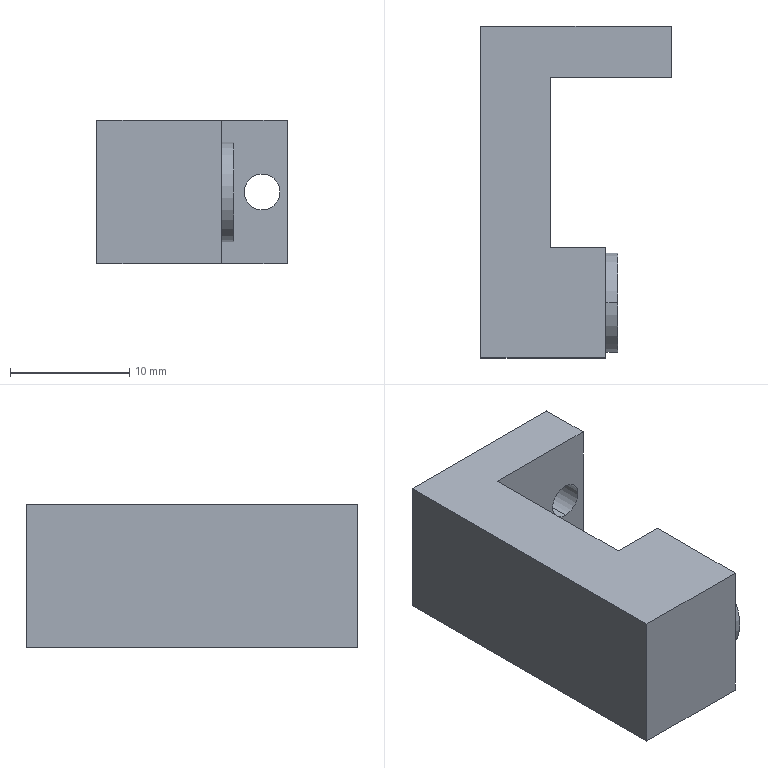Part | SolidWorks | features SavedExtBody 1 | 1 solid | 21 faces | box 15.948 x 27.791 x 12 mm | volume 2925 mm3 | plane 11 | cylinder 8 | cone 2 | commonest cylinder face diameters 3 x4 4.217 x2 8.358 x2
STEP:
#1=CARTESIAN_POINT('',(81.489,-181.285,66.5));
#2=VERTEX_POINT('',#1);
#3=CARTESIAN_POINT('',(81.489,-181.285,63.5));
#4=VERTEX_POINT('',#3);
#5=CARTESIAN_POINT('',(81.489,-181.285,65.));
#6=DIRECTION('',(0.,-1.,0.));
#7=DIRECTION('',(0.,0.,-1.));
#8=AXIS2_PLACEMENT_3D('',#5,#6,#7);
#9=CIRCLE('',#8,1.5);
#10=EDGE_CURVE('',#2,#4,#9,.T.);
#11=ORIENTED_EDGE('',*,*,#10,.F.);
#12=CARTESIAN_POINT('',(81.489,-185.569,66.5));
#13=VERTEX_POINT('',#12);
#14=CARTESIAN_POINT('',(81.489,-163.569,66.5));
#15=DIRECTION('',(0.,-1.,0.));
#16=VECTOR('',#15,1000.);
#17=LINE('',#14,#16);
#18=EDGE_CURVE('',#2,#13,#17,.T.);
#19=ORIENTED_EDGE('',*,*,#18,.T.);
#20=CARTESIAN_POINT('',(81.489,-185.569,63.5));
#21=VERTEX_POINT('',#20);
#22=CARTESIAN_POINT('',(81.489,-185.569,65.));
#23=DIRECTION('',(0.,-1.,0.));
#24=DIRECTION('',(0.,0.,-1.));
#25=AXIS2_PLACEMENT_3D('',#22,#23,#24);
#26=CIRCLE('',#25,1.5);
#27=EDGE_CURVE('',#13,#21,#26,.T.);
#28=ORIENTED_EDGE('',*,*,#27,.T.);
#29=CARTESIAN_POINT('',(81.489,-163.569,63.5));
#30=DIRECTION('',(0.,-1.,0.));
#31=VECTOR('',#30,1000.);
#32=LINE('',#29,#31);
#33=EDGE_CURVE('',#4,#21,#32,.T.);
#34=ORIENTED_EDGE('',*,*,#33,.F.);
#35=EDGE_LOOP('',(#11,#19,#28,#34));
#36=FACE_OUTER_BOUND('',#35,.T.);
#37=CARTESIAN_POINT('',(81.489,-163.569,65.));
#38=DIRECTION('',(0.,-1.,0.));
#39=DIRECTION('',(0.,0.,-1.));
#40=AXIS2_PLACEMENT_3D('',#37,#38,#39);
#41=CYLINDRICAL_SURFACE('',#40,1.5);
#42=ADVANCED_FACE('',(#36),#41,.F.);
#43=CARTESIAN_POINT('',(87.424,-181.285,66.5));
#44=VERTEX_POINT('',#43);
#45=CARTESIAN_POINT('',(87.424,-181.285,63.5));
#46=VERTEX_POINT('',#45);
#47=CARTESIAN_POINT('',(87.424,-181.285,65.));
#48=DIRECTION('',(0.,-1.,0.));
#49=DIRECTION('',(0.,0.,-1.));
#50=AXIS2_PLACEMENT_3D('',#47,#48,#49);
#51=CIRCLE('',#50,1.5);
#52=EDGE_CURVE('',#44,#46,#51,.T.);
#53=ORIENTED_EDGE('',*,*,#52,.F.);
#54=CARTESIAN_POINT('',(87.424,-185.569,66.5));
#55=VERTEX_POINT('',#54);
#56=CARTESIAN_POINT('',(87.424,-163.569,66.5));
#57=DIRECTION('',(0.,-1.,0.));
#58=VECTOR('',#57,1000.);
#59=LINE('',#56,#58);
#60=EDGE_CURVE('',#44,#55,#59,.T.);
#61=ORIENTED_EDGE('',*,*,#60,.T.);
#62=CARTESIAN_POINT('',(87.424,-185.569,63.5));
#63=VERTEX_POINT('',#62);
#64=CARTESIAN_POINT('',(87.424,-185.569,65.));
#65=DIRECTION('',(0.,-1.,0.));
#66=DIRECTION('',(0.,0.,1.));
#67=AXIS2_PLACEMENT_3D('',#64,#65,#66);
#68=CIRCLE('',#67,1.5);
#69=EDGE_CURVE('',#55,#63,#68,.T.);
#70=ORIENTED_EDGE('',*,*,#69,.T.);
#71=CARTESIAN_POINT('',(87.424,-163.569,63.5));
#72=DIRECTION('',(0.,-1.,0.));
#73=VECTOR('',#72,1000.);
#74=LINE('',#71,#73);
#75=EDGE_CURVE('',#46,#63,#74,.T.);
#76=ORIENTED_EDGE('',*,*,#75,.F.);
#77=EDGE_LOOP('',(#53,#61,#70,#76));
#78=FACE_OUTER_BOUND('',#77,.T.);
#79=CARTESIAN_POINT('',(87.424,-163.569,65.));
#80=DIRECTION('',(0.,-1.,0.));
#81=DIRECTION('',(0.,0.,-1.));
#82=AXIS2_PLACEMENT_3D('',#79,#80,#81);
#83=CYLINDRICAL_SURFACE('',#82,1.5);
#84=ADVANCED_FACE('',(#78),#83,.F.);
#85=CARTESIAN_POINT('',(78.287,-204.466,65.));
#86=VERTEX_POINT('',#85);
#87=CARTESIAN_POINT('',(83.675,-204.466,62.892));
#88=VERTEX_POINT('',#87);
#89=CARTESIAN_POINT('',(83.675,-204.466,62.892));
#90=DIRECTION('',(0.9312,0.,-0.3644));
#91=VECTOR('',#90,1000.);
#92=LINE('',#89,#91);
#93=EDGE_CURVE('',#86,#88,#92,.T.);
#94=ORIENTED_EDGE('',*,*,#93,.F.);
#95=CARTESIAN_POINT('',(83.675,-204.466,67.108));
#96=VERTEX_POINT('',#95);
#97=CARTESIAN_POINT('',(83.675,-204.466,67.108));
#98=DIRECTION('',(0.9312,0.,0.3644));
#99=VECTOR('',#98,1000.);
#100=LINE('',#97,#99);
#101=EDGE_CURVE('',#86,#96,#100,.T.);
#102=ORIENTED_EDGE('',*,*,#101,.T.);
#103=CARTESIAN_POINT('',(83.675,-204.466,65.));
#104=DIRECTION('',(1.,0.,0.));
#105=DIRECTION('',(0.,0.,-1.));
#106=AXIS2_PLACEMENT_3D('',#103,#104,#105);
#107=CIRCLE('',#106,2.108);
#108=EDGE_CURVE('',#96,#88,#107,.T.);
#109=ORIENTED_EDGE('',*,*,#108,.T.);
#110=EDGE_LOOP('',(#94,#102,#109));
#111=FACE_OUTER_BOUND('',#110,.T.);
#112=CARTESIAN_POINT('',(83.675,-204.466,65.));
#113=DIRECTION('',(1.,0.,0.));
#114=DIRECTION('',(0.,0.,-1.));
#115=AXIS2_PLACEMENT_3D('',#112,#113,#114);
#116=CONICAL_SURFACE('',#115,2.108,0.373);
#117=ADVANCED_FACE('',(#111),#116,.F.);
#118=ORIENTED_EDGE('',*,*,#108,.F.);
#119=CARTESIAN_POINT('',(85.041,-204.466,67.108));
#120=VERTEX_POINT('',#119);
#121=CARTESIAN_POINT('',(100.386,-204.466,67.108));
#122=DIRECTION('',(1.,0.,0.));
#123=VECTOR('',#122,1000.);
#124=LINE('',#121,#123);
#125=EDGE_CURVE('',#96,#120,#124,.T.);
#126=ORIENTED_EDGE('',*,*,#125,.T.);
#127=CARTESIAN_POINT('',(85.041,-204.466,62.892));
#128=VERTEX_POINT('',#127);
#129=CARTESIAN_POINT('',(85.041,-204.466,65.));
#130=DIRECTION('',(1.,0.,0.));
#131=DIRECTION('',(0.,0.,-1.));
#132=AXIS2_PLACEMENT_3D('',#129,#130,#131);
#133=CIRCLE('',#132,2.108);
#134=EDGE_CURVE('',#120,#128,#133,.T.);
#135=ORIENTED_EDGE('',*,*,#134,.T.);
#136=CARTESIAN_POINT('',(100.386,-204.466,62.892));
#137=DIRECTION('',(1.,0.,0.));
#138=VECTOR('',#137,1000.);
#139=LINE('',#136,#138);
#140=EDGE_CURVE('',#88,#128,#139,.T.);
#141=ORIENTED_EDGE('',*,*,#140,.F.);
#142=EDGE_LOOP('',(#118,#126,#135,#141));
#143=FACE_OUTER_BOUND('',#142,.T.);
#144=CARTESIAN_POINT('',(100.386,-204.466,65.));
#145=DIRECTION('',(1.,0.,0.));
#146=DIRECTION('',(0.,0.,-1.));
#147=AXIS2_PLACEMENT_3D('',#144,#145,#146);
#148=CYLINDRICAL_SURFACE('',#147,2.108);
#149=ADVANCED_FACE('',(#143),#148,.F.);
#150=CARTESIAN_POINT('',(85.041,-204.466,60.821));
#151=VERTEX_POINT('',#150);
#152=CARTESIAN_POINT('',(85.041,-204.466,69.179));
#153=VERTEX_POINT('',#152);
#154=CARTESIAN_POINT('',(85.041,-204.466,65.));
#155=DIRECTION('',(1.,0.,0.));
#156=DIRECTION('',(0.,0.,-1.));
#157=AXIS2_PLACEMENT_3D('',#154,#155,#156);
#158=CIRCLE('',#157,4.179);
#159=EDGE_CURVE('',#151,#153,#158,.T.);
#160=ORIENTED_EDGE('',*,*,#159,.F.);
#161=CARTESIAN_POINT('',(84.041,-204.466,60.821));
#162=VERTEX_POINT('',#161);
#163=CARTESIAN_POINT('',(85.041,-204.466,60.821));
#164=DIRECTION('',(-1.,0.,0.));
#165=VECTOR('',#164,1000.);
#166=LINE('',#163,#165);
#167=EDGE_CURVE('',#151,#162,#166,.T.);
#168=ORIENTED_EDGE('',*,*,#167,.T.);
#169=CARTESIAN_POINT('',(84.041,-204.466,69.179));
#170=VERTEX_POINT('',#169);
#171=CARTESIAN_POINT('',(84.041,-204.466,65.));
#172=DIRECTION('',(1.,0.,0.));
#173=DIRECTION('',(0.,0.,-1.));
#174=AXIS2_PLACEMENT_3D('',#171,#172,#173);
#175=CIRCLE('',#174,4.179);
#176=EDGE_CURVE('',#162,#170,#175,.T.);
#177=ORIENTED_EDGE('',*,*,#176,.T.);
#178=CARTESIAN_POINT('',(85.041,-204.466,69.179));
#179=DIRECTION('',(-1.,0.,0.));
#180=VECTOR('',#179,1000.);
#181=LINE('',#178,#180);
#182=EDGE_CURVE('',#153,#170,#181,.T.);
#183=ORIENTED_EDGE('',*,*,#182,.F.);
#184=EDGE_LOOP('',(#160,#168,#177,#183));
#185=FACE_OUTER_BOUND('',#184,.T.);
#186=CARTESIAN_POINT('',(85.041,-204.466,65.));
#187=DIRECTION('',(-1.,0.,0.));
#188=DIRECTION('',(0.,0.,1.));
#189=AXIS2_PLACEMENT_3D('',#186,#187,#188);
#190=CYLINDRICAL_SURFACE('',#189,4.179);
#191=ADVANCED_FACE('',(#185),#190,.T.);
#192=CARTESIAN_POINT('',(84.041,-199.856,59.));
#193=VERTEX_POINT('',#192);
#194=CARTESIAN_POINT('',(79.389,-199.856,59.));
#195=VERTEX_POINT('',#194);
#196=CARTESIAN_POINT('',(0.,-199.856,59.));
#197=DIRECTION('',(-1.,0.,0.));
#198=VECTOR('',#197,1000.);
#199=LINE('',#196,#198);
#200=EDGE_CURVE('',#193,#195,#199,.T.);
#201=ORIENTED_EDGE('',*,*,#200,.T.);
#202=CARTESIAN_POINT('',(79.389,-199.856,71.));
#203=VERTEX_POINT('',#202);
#204=CARTESIAN_POINT('',(79.389,-199.856,71.));
#205=DIRECTION('',(0.,0.,-1.));
#206=VECTOR('',#205,1000.);
#207=LINE('',#204,#206);
#208=EDGE_CURVE('',#203,#195,#207,.T.);
#209=ORIENTED_EDGE('',*,*,#208,.F.);
#210=CARTESIAN_POINT('',(84.041,-199.856,71.));
#211=VERTEX_POINT('',#210);
#212=CARTESIAN_POINT('',(0.,-199.856,71.));
#213=DIRECTION('',(-1.,0.,0.));
#214=VECTOR('',#213,1000.);
#215=LINE('',#212,#214);
#216=EDGE_CURVE('',#211,#203,#215,.T.);
#217=ORIENTED_EDGE('',*,*,#216,.F.);
#218=CARTESIAN_POINT('',(84.041,-199.856,71.));
#219=DIRECTION('',(0.,0.,-1.));
#220=VECTOR('',#219,1000.);
#221=LINE('',#218,#220);
#222=EDGE_CURVE('',#211,#193,#221,.T.);
#223=ORIENTED_EDGE('',*,*,#222,.T.);
#224=EDGE_LOOP('',(#201,#209,#217,#223));
#225=FACE_OUTER_BOUND('',#224,.T.);
#226=CARTESIAN_POINT('',(0.,-199.856,71.));
#227=DIRECTION('',(0.,-1.,0.));
#228=DIRECTION('',(0.,0.,-1.));
#229=AXIS2_PLACEMENT_3D('',#226,#227,#228);
#230=PLANE('',#229);
#231=ADVANCED_FACE('',(#225),#230,.F.);
#232=CARTESIAN_POINT('',(79.389,-185.569,59.));
#233=VERTEX_POINT('',#232);
#234=CARTESIAN_POINT('',(79.389,0.,59.));
#235=DIRECTION('',(0.,1.,0.));
#236=VECTOR('',#235,1000.);
#237=LINE('',#234,#236);
#238=EDGE_CURVE('',#195,#233,#237,.T.);
#239=ORIENTED_EDGE('',*,*,#238,.T.);
#240=CARTESIAN_POINT('',(79.389,-185.569,71.));
#241=VERTEX_POINT('',#240);
#242=CARTESIAN_POINT('',(79.389,-185.569,71.));
#243=DIRECTION('',(0.,0.,-1.));
#244=VECTOR('',#243,1000.);
#245=LINE('',#242,#244);
#246=EDGE_CURVE('',#241,#233,#245,.T.);
#247=ORIENTED_EDGE('',*,*,#246,.F.);
#248=CARTESIAN_POINT('',(79.389,0.,71.));
#249=DIRECTION('',(0.,1.,0.));
#250=VECTOR('',#249,1000.);
#251=LINE('',#248,#250);
#252=EDGE_CURVE('',#203,#241,#251,.T.);
#253=ORIENTED_EDGE('',*,*,#252,.F.);
#254=ORIENTED_EDGE('',*,*,#208,.T.);
#255=EDGE_LOOP('',(#239,#247,#253,#254));
#256=FACE_OUTER_BOUND('',#255,.T.);
#257=CARTESIAN_POINT('',(79.389,0.,71.));
#258=DIRECTION('',(-1.,0.,0.));
#259=DIRECTION('',(0.,0.,1.));
#260=AXIS2_PLACEMENT_3D('',#257,#258,#259);
#261=PLANE('',#260);
#262=ADVANCED_FACE('',(#256),#261,.F.);
#263=CARTESIAN_POINT('',(81.489,-185.569,65.));
#264=DIRECTION('',(0.,-1.,0.));
#265=DIRECTION('',(0.,0.,-1.));
#266=AXIS2_PLACEMENT_3D('',#263,#264,#265);
#267=CIRCLE('',#266,1.5);
#268=EDGE_CURVE('',#21,#13,#267,.T.);
#269=ORIENTED_EDGE('',*,*,#268,.F.);
#270=ORIENTED_EDGE('',*,*,#27,.F.);
#271=EDGE_LOOP('',(#269,#270));
#272=FACE_BOUND('',#271,.T.);
#273=CARTESIAN_POINT('',(87.424,-185.569,65.));
#274=DIRECTION('',(0.,-1.,0.));
#275=DIRECTION('',(0.,0.,1.));
#276=AXIS2_PLACEMENT_3D('',#273,#274,#275);
#277=CIRCLE('',#276,1.5);
#278=EDGE_CURVE('',#63,#55,#277,.T.);
#279=ORIENTED_EDGE('',*,*,#278,.F.);
#280=ORIENTED_EDGE('',*,*,#69,.F.);
#281=EDGE_LOOP('',(#279,#280));
#282=FACE_BOUND('',#281,.T.);
#283=CARTESIAN_POINT('',(89.523,-185.569,59.));
#284=VERTEX_POINT('',#283);
#285=CARTESIAN_POINT('',(0.,-185.569,59.));
#286=DIRECTION('',(-1.,0.,0.));
#287=VECTOR('',#286,1000.);
#288=LINE('',#285,#287);
#289=EDGE_CURVE('',#284,#233,#288,.T.);
#290=ORIENTED_EDGE('',*,*,#289,.F.);
#291=CARTESIAN_POINT('',(89.523,-185.569,71.));
#292=VERTEX_POINT('',#291);
#293=CARTESIAN_POINT('',(89.523,-185.569,71.));
#294=DIRECTION('',(0.,0.,-1.));
#295=VECTOR('',#294,1000.);
#296=LINE('',#293,#295);
#297=EDGE_CURVE('',#292,#284,#296,.T.);
#298=ORIENTED_EDGE('',*,*,#297,.F.);
#299=CARTESIAN_POINT('',(0.,-185.569,71.));
#300=DIRECTION('',(-1.,0.,0.));
#301=VECTOR('',#300,1000.);
#302=LINE('',#299,#301);
#303=EDGE_CURVE('',#292,#241,#302,.T.);
#304=ORIENTED_EDGE('',*,*,#303,.T.);
#305=ORIENTED_EDGE('',*,*,#246,.T.);
#306=EDGE_LOOP('',(#290,#298,#304,#305));
#307=FACE_OUTER_BOUND('',#306,.T.);
#308=CARTESIAN_POINT('',(0.,-185.569,71.));
#309=DIRECTION('',(0.,-1.,0.));
#310=DIRECTION('',(0.,0.,-1.));
#311=AXIS2_PLACEMENT_3D('',#308,#309,#310);
#312=PLANE('',#311);
#313=ADVANCED_FACE('',(#272,#282,#307),#312,.T.);
#314=CARTESIAN_POINT('',(89.523,-181.285,59.));
#315=VERTEX_POINT('',#314);
#316=CARTESIAN_POINT('',(89.523,0.,59.));
#317=DIRECTION('',(0.,-1.,0.));
#318=VECTOR('',#317,1000.);
#319=LINE('',#316,#318);
#320=EDGE_CURVE('',#315,#284,#319,.T.);
#321=ORIENTED_EDGE('',*,*,#320,.F.);
#322=CARTESIAN_POINT('',(89.523,-181.285,71.));
#323=VERTEX_POINT('',#322);
#324=CARTESIAN_POINT('',(89.523,-181.285,71.));
#325=DIRECTION('',(0.,0.,-1.));
#326=VECTOR('',#325,1000.);
#327=LINE('',#324,#326);
#328=EDGE_CURVE('',#323,#315,#327,.T.);
#329=ORIENTED_EDGE('',*,*,#328,.F.);
#330=CARTESIAN_POINT('',(89.523,0.,71.));
#331=DIRECTION('',(0.,-1.,0.));
#332=VECTOR('',#331,1000.);
#333=LINE('',#330,#332);
#334=EDGE_CURVE('',#323,#292,#333,.T.);
#335=ORIENTED_EDGE('',*,*,#334,.T.);
#336=ORIENTED_EDGE('',*,*,#297,.T.);
#337=EDGE_LOOP('',(#321,#329,#335,#336));
#338=FACE_OUTER_BOUND('',#337,.T.);
#339=CARTESIAN_POINT('',(89.523,0.,71.));
#340=DIRECTION('',(1.,0.,0.));
#341=DIRECTION('',(0.,0.,-1.));
#342=AXIS2_PLACEMENT_3D('',#339,#340,#341);
#343=PLANE('',#342);
#344=ADVANCED_FACE('',(#338),#343,.T.);
#345=CARTESIAN_POINT('',(81.489,-181.285,65.));
#346=DIRECTION('',(0.,-1.,0.));
#347=DIRECTION('',(0.,0.,-1.));
#348=AXIS2_PLACEMENT_3D('',#345,#346,#347);
#349=CIRCLE('',#348,1.5);
#350=EDGE_CURVE('',#4,#2,#349,.T.);
#351=ORIENTED_EDGE('',*,*,#350,.T.);
#352=ORIENTED_EDGE('',*,*,#10,.T.);
#353=EDGE_LOOP('',(#351,#352));
#354=FACE_BOUND('',#353,.T.);
#355=CARTESIAN_POINT('',(87.424,-181.285,65.));
#356=DIRECTION('',(0.,-1.,0.));
#357=DIRECTION('',(0.,0.,-1.));
#358=AXIS2_PLACEMENT_3D('',#355,#356,#357);
#359=CIRCLE('',#358,1.5);
#360=EDGE_CURVE('',#46,#44,#359,.T.);
#361=ORIENTED_EDGE('',*,*,#360,.T.);
#362=ORIENTED_EDGE('',*,*,#52,.T.);
#363=EDGE_LOOP('',(#361,#362));
#364=FACE_BOUND('',#363,.T.);
#365=CARTESIAN_POINT('',(73.575,-181.285,59.));
#366=VERTEX_POINT('',#365);
#367=CARTESIAN_POINT('',(0.,-181.285,59.));
#368=DIRECTION('',(-1.,0.,0.));
#369=VECTOR('',#368,1000.);
#370=LINE('',#367,#369);
#371=EDGE_CURVE('',#315,#366,#370,.T.);
#372=ORIENTED_EDGE('',*,*,#371,.T.);
#373=CARTESIAN_POINT('',(73.575,-181.285,71.));
#374=VERTEX_POINT('',#373);
#375=CARTESIAN_POINT('',(73.575,-181.285,71.));
#376=DIRECTION('',(0.,0.,-1.));
#377=VECTOR('',#376,1000.);
#378=LINE('',#375,#377);
#379=EDGE_CURVE('',#374,#366,#378,.T.);
#380=ORIENTED_EDGE('',*,*,#379,.F.);
#381=CARTESIAN_POINT('',(0.,-181.285,71.));
#382=DIRECTION('',(-1.,0.,0.));
#383=VECTOR('',#382,1000.);
#384=LINE('',#381,#383);
#385=EDGE_CURVE('',#323,#374,#384,.T.);
#386=ORIENTED_EDGE('',*,*,#385,.F.);
#387=ORIENTED_EDGE('',*,*,#328,.T.);
#388=EDGE_LOOP('',(#372,#380,#386,#387));
#389=FACE_OUTER_BOUND('',#388,.T.);
#390=CARTESIAN_POINT('',(0.,-181.285,71.));
#391=DIRECTION('',(0.,-1.,0.));
#392=DIRECTION('',(0.,0.,-1.));
#393=AXIS2_PLACEMENT_3D('',#390,#391,#392);
#394=PLANE('',#393);
#395=ADVANCED_FACE('',(#354,#364,#389),#394,.F.);
#396=CARTESIAN_POINT('',(73.575,-209.076,59.));
#397=VERTEX_POINT('',#396);
#398=CARTESIAN_POINT('',(73.575,0.,59.));
#399=DIRECTION('',(0.,-1.,0.));
#400=VECTOR('',#399,1000.);
#401=LINE('',#398,#400);
#402=EDGE_CURVE('',#366,#397,#401,.T.);
#403=ORIENTED_EDGE('',*,*,#402,.T.);
#404=CARTESIAN_POINT('',(73.575,-209.076,71.));
#405=VERTEX_POINT('',#404);
#406=CARTESIAN_POINT('',(73.575,-209.076,71.));
#407=DIRECTION('',(0.,0.,-1.));
#408=VECTOR('',#407,1000.);
#409=LINE('',#406,#408);
#410=EDGE_CURVE('',#405,#397,#409,.T.);
#411=ORIENTED_EDGE('',*,*,#410,.F.);
#412=CARTESIAN_POINT('',(73.575,0.,71.));
#413=DIRECTION('',(0.,-1.,0.));
#414=VECTOR('',#413,1000.);
#415=LINE('',#412,#414);
#416=EDGE_CURVE('',#374,#405,#415,.T.);
#417=ORIENTED_EDGE('',*,*,#416,.F.);
#418=ORIENTED_EDGE('',*,*,#379,.T.);
#419=EDGE_LOOP('',(#403,#411,#417,#418));
#420=FACE_OUTER_BOUND('',#419,.T.);
#421=CARTESIAN_POINT('',(73.575,0.,71.));
#422=DIRECTION('',(1.,0.,0.));
#423=DIRECTION('',(0.,0.,-1.));
#424=AXIS2_PLACEMENT_3D('',#421,#422,#423);
#425=PLANE('',#424);
#426=ADVANCED_FACE('',(#420),#425,.F.);
#427=CARTESIAN_POINT('',(84.041,-209.076,59.));
#428=VERTEX_POINT('',#427);
#429=CARTESIAN_POINT('',(0.,-209.076,59.));
#430=DIRECTION('',(1.,0.,0.));
#431=VECTOR('',#430,1000.);
#432=LINE('',#429,#431);
#433=EDGE_CURVE('',#397,#428,#432,.T.);
#434=ORIENTED_EDGE('',*,*,#433,.T.);
#435=CARTESIAN_POINT('',(84.041,-209.076,71.));
#436=VERTEX_POINT('',#435);
#437=CARTESIAN_POINT('',(84.041,-209.076,71.));
#438=DIRECTION('',(0.,0.,-1.));
#439=VECTOR('',#438,1000.);
#440=LINE('',#437,#439);
#441=EDGE_CURVE('',#436,#428,#440,.T.);
#442=ORIENTED_EDGE('',*,*,#441,.F.);
#443=CARTESIAN_POINT('',(0.,-209.076,71.));
#444=DIRECTION('',(1.,0.,0.));
#445=VECTOR('',#444,1000.);
#446=LINE('',#443,#445);
#447=EDGE_CURVE('',#405,#436,#446,.T.);
#448=ORIENTED_EDGE('',*,*,#447,.F.);
#449=ORIENTED_EDGE('',*,*,#410,.T.);
#450=EDGE_LOOP('',(#434,#442,#448,#449));
#451=FACE_OUTER_BOUND('',#450,.T.);
#452=CARTESIAN_POINT('',(0.,-209.076,71.));
#453=DIRECTION('',(0.,1.,0.));
#454=DIRECTION('',(0.,0.,1.));
#455=AXIS2_PLACEMENT_3D('',#452,#453,#454);
#456=PLANE('',#455);
#457=ADVANCED_FACE('',(#451),#456,.F.);
#458=CARTESIAN_POINT('',(84.041,-204.466,65.));
#459=DIRECTION('',(1.,0.,0.));
#460=DIRECTION('',(0.,0.,-1.));
#461=AXIS2_PLACEMENT_3D('',#458,#459,#460);
#462=CIRCLE('',#461,4.179);
#463=EDGE_CURVE('',#170,#162,#462,.T.);
#464=ORIENTED_EDGE('',*,*,#463,.F.);
#465=ORIENTED_EDGE('',*,*,#176,.F.);
#466=EDGE_LOOP('',(#464,#465));
#467=FACE_BOUND('',#466,.T.);
#468=CARTESIAN_POINT('',(84.041,0.,59.));
#469=DIRECTION('',(0.,-1.,0.));
#470=VECTOR('',#469,1000.);
#471=LINE('',#468,#470);
#472=EDGE_CURVE('',#193,#428,#471,.T.);
#473=ORIENTED_EDGE('',*,*,#472,.F.);
#474=ORIENTED_EDGE('',*,*,#222,.F.);
#475=CARTESIAN_POINT('',(84.041,0.,71.));
#476=DIRECTION('',(0.,-1.,0.));
#477=VECTOR('',#476,1000.);
#478=LINE('',#475,#477);
#479=EDGE_CURVE('',#211,#436,#478,.T.);
#480=ORIENTED_EDGE('',*,*,#479,.T.);
#481=ORIENTED_EDGE('',*,*,#441,.T.);
#482=EDGE_LOOP('',(#473,#474,#480,#481));
#483=FACE_OUTER_BOUND('',#482,.T.);
#484=CARTESIAN_POINT('',(84.041,0.,71.));
#485=DIRECTION('',(1.,0.,0.));
#486=DIRECTION('',(0.,0.,-1.));
#487=AXIS2_PLACEMENT_3D('',#484,#485,#486);
#488=PLANE('',#487);
#489=ADVANCED_FACE('',(#467,#483),#488,.T.);
#490=ORIENTED_EDGE('',*,*,#216,.T.);
#491=ORIENTED_EDGE('',*,*,#252,.T.);
#492=ORIENTED_EDGE('',*,*,#303,.F.);
#493=ORIENTED_EDGE('',*,*,#334,.F.);
#494=ORIENTED_EDGE('',*,*,#385,.T.);
#495=ORIENTED_EDGE('',*,*,#416,.T.);
#496=ORIENTED_EDGE('',*,*,#447,.T.);
#497=ORIENTED_EDGE('',*,*,#479,.F.);
#498=EDGE_LOOP('',(#490,#491,#492,#493,#494,#495,#496,#497));
#499=FACE_OUTER_BOUND('',#498,.T.);
#500=CARTESIAN_POINT('',(0.,0.,71.));
#501=DIRECTION('',(0.,0.,1.));
#502=DIRECTION('',(1.,0.,0.));
#503=AXIS2_PLACEMENT_3D('',#500,#501,#502);
#504=PLANE('',#503);
#505=ADVANCED_FACE('',(#499),#504,.T.);
#506=ORIENTED_EDGE('',*,*,#200,.F.);
#507=ORIENTED_EDGE('',*,*,#472,.T.);
#508=ORIENTED_EDGE('',*,*,#433,.F.);
#509=ORIENTED_EDGE('',*,*,#402,.F.);
#510=ORIENTED_EDGE('',*,*,#371,.F.);
#511=ORIENTED_EDGE('',*,*,#320,.T.);
#512=ORIENTED_EDGE('',*,*,#289,.T.);
#513=ORIENTED_EDGE('',*,*,#238,.F.);
#514=EDGE_LOOP('',(#506,#507,#508,#509,#510,#511,#512,#513));
#515=FACE_OUTER_BOUND('',#514,.T.);
#516=CARTESIAN_POINT('',(0.,0.,59.));
#517=DIRECTION('',(0.,0.,1.));
#518=DIRECTION('',(1.,0.,0.));
#519=AXIS2_PLACEMENT_3D('',#516,#517,#518);
#520=PLANE('',#519);
#521=ADVANCED_FACE('',(#515),#520,.F.);
#522=ORIENTED_EDGE('',*,*,#167,.F.);
#523=CARTESIAN_POINT('',(85.041,-204.466,65.));
#524=DIRECTION('',(1.,0.,0.));
#525=DIRECTION('',(0.,0.,-1.));
#526=AXIS2_PLACEMENT_3D('',#523,#524,#525);
#527=CIRCLE('',#526,4.179);
#528=EDGE_CURVE('',#153,#151,#527,.T.);
#529=ORIENTED_EDGE('',*,*,#528,.F.);
#530=ORIENTED_EDGE('',*,*,#182,.T.);
#531=ORIENTED_EDGE('',*,*,#463,.T.);
#532=EDGE_LOOP('',(#522,#529,#530,#531));
#533=FACE_OUTER_BOUND('',#532,.T.);
#534=CARTESIAN_POINT('',(85.041,-204.466,65.));
#535=DIRECTION('',(-1.,0.,0.));
#536=DIRECTION('',(0.,0.,1.));
#537=AXIS2_PLACEMENT_3D('',#534,#535,#536);
#538=CYLINDRICAL_SURFACE('',#537,4.179);
#539=ADVANCED_FACE('',(#533),#538,.T.);
#540=CARTESIAN_POINT('',(85.041,-204.466,65.));
#541=DIRECTION('',(1.,0.,0.));
#542=DIRECTION('',(0.,0.,-1.));
#543=AXIS2_PLACEMENT_3D('',#540,#541,#542);
#544=CIRCLE('',#543,2.108);
#545=EDGE_CURVE('',#128,#120,#544,.T.);
#546=ORIENTED_EDGE('',*,*,#545,.F.);
#547=ORIENTED_EDGE('',*,*,#134,.F.);
#548=EDGE_LOOP('',(#546,#547));
#549=FACE_BOUND('',#548,.T.);
#550=ORIENTED_EDGE('',*,*,#528,.T.);
#551=ORIENTED_EDGE('',*,*,#159,.T.);
#552=EDGE_LOOP('',(#550,#551));
#553=FACE_OUTER_BOUND('',#552,.T.);
#554=CARTESIAN_POINT('',(85.041,-204.466,65.));
#555=DIRECTION('',(1.,0.,0.));
#556=DIRECTION('',(0.,0.,-1.));
#557=AXIS2_PLACEMENT_3D('',#554,#555,#556);
#558=PLANE('',#557);
#559=ADVANCED_FACE('',(#549,#553),#558,.T.);
#560=ORIENTED_EDGE('',*,*,#125,.F.);
#561=CARTESIAN_POINT('',(83.675,-204.466,65.));
#562=DIRECTION('',(1.,0.,0.));
#563=DIRECTION('',(0.,0.,-1.));
#564=AXIS2_PLACEMENT_3D('',#561,#562,#563);
#565=CIRCLE('',#564,2.108);
#566=EDGE_CURVE('',#88,#96,#565,.T.);
#567=ORIENTED_EDGE('',*,*,#566,.F.);
#568=ORIENTED_EDGE('',*,*,#140,.T.);
#569=ORIENTED_EDGE('',*,*,#545,.T.);
#570=EDGE_LOOP('',(#560,#567,#568,#569));
#571=FACE_OUTER_BOUND('',#570,.T.);
#572=CARTESIAN_POINT('',(100.386,-204.466,65.));
#573=DIRECTION('',(1.,0.,0.));
#574=DIRECTION('',(0.,0.,-1.));
#575=AXIS2_PLACEMENT_3D('',#572,#573,#574);
#576=CYLINDRICAL_SURFACE('',#575,2.108);
#577=ADVANCED_FACE('',(#571),#576,.F.);
#578=ORIENTED_EDGE('',*,*,#101,.F.);
#579=ORIENTED_EDGE('',*,*,#93,.T.);
#580=ORIENTED_EDGE('',*,*,#566,.T.);
#581=EDGE_LOOP('',(#578,#579,#580));
#582=FACE_OUTER_BOUND('',#581,.T.);
#583=CARTESIAN_POINT('',(83.675,-204.466,65.));
#584=DIRECTION('',(1.,0.,0.));
#585=DIRECTION('',(0.,0.,-1.));
#586=AXIS2_PLACEMENT_3D('',#583,#584,#585);
#587=CONICAL_SURFACE('',#586,2.108,0.373);
#588=ADVANCED_FACE('',(#582),#587,.F.);
#589=ORIENTED_EDGE('',*,*,#60,.F.);
#590=ORIENTED_EDGE('',*,*,#360,.F.);
#591=ORIENTED_EDGE('',*,*,#75,.T.);
#592=ORIENTED_EDGE('',*,*,#278,.T.);
#593=EDGE_LOOP('',(#589,#590,#591,#592));
#594=FACE_OUTER_BOUND('',#593,.T.);
#595=CARTESIAN_POINT('',(87.424,-163.569,65.));
#596=DIRECTION('',(0.,-1.,0.));
#597=DIRECTION('',(0.,0.,-1.));
#598=AXIS2_PLACEMENT_3D('',#595,#596,#597);
#599=CYLINDRICAL_SURFACE('',#598,1.5);
#600=ADVANCED_FACE('',(#594),#599,.F.);
#601=ORIENTED_EDGE('',*,*,#18,.F.);
#602=ORIENTED_EDGE('',*,*,#350,.F.);
#603=ORIENTED_EDGE('',*,*,#33,.T.);
#604=ORIENTED_EDGE('',*,*,#268,.T.);
#605=EDGE_LOOP('',(#601,#602,#603,#604));
#606=FACE_OUTER_BOUND('',#605,.T.);
#607=CARTESIAN_POINT('',(81.489,-163.569,65.));
#608=DIRECTION('',(0.,-1.,0.));
#609=DIRECTION('',(0.,0.,-1.));
#610=AXIS2_PLACEMENT_3D('',#607,#608,#609);
#611=CYLINDRICAL_SURFACE('',#610,1.5);
#612=ADVANCED_FACE('',(#606),#611,.F.);
#613=CLOSED_SHELL('',(#42,#84,#117,#149,#191,#231,#262,#313,#344,#395,#426,#457,#489,#505,#521,#539,#559,#577,#588,#600,#612));
#614=MANIFOLD_SOLID_BREP('',#613);
#615=CARTESIAN_POINT('',(0.,0.,0.));
#616=DIRECTION('',(0.,0.,1.));
#617=DIRECTION('',(1.,0.,0.));
#618=AXIS2_PLACEMENT_3D('',#615,#616,#617);
#619=(LENGTH_UNIT()NAMED_UNIT(*)SI_UNIT(.MILLI.,.METRE.));
#620=UNCERTAINTY_MEASURE_WITH_UNIT(LENGTH_MEASURE(0.00001),#619,'','');
#621=(NAMED_UNIT(*)PLANE_ANGLE_UNIT()SI_UNIT($,.RADIAN.));
#622=(NAMED_UNIT(*)SI_UNIT($,.STERADIAN.)SOLID_ANGLE_UNIT());
#623=(GEOMETRIC_REPRESENTATION_CONTEXT(3)GLOBAL_UNCERTAINTY_ASSIGNED_CONTEXT((#620))GLOBAL_UNIT_ASSIGNED_CONTEXT((#619,#621,#622))REPRESENTATION_CONTEXT('',''));
#624=ADVANCED_BREP_SHAPE_REPRESENTATION('',(#614,#618),#623);